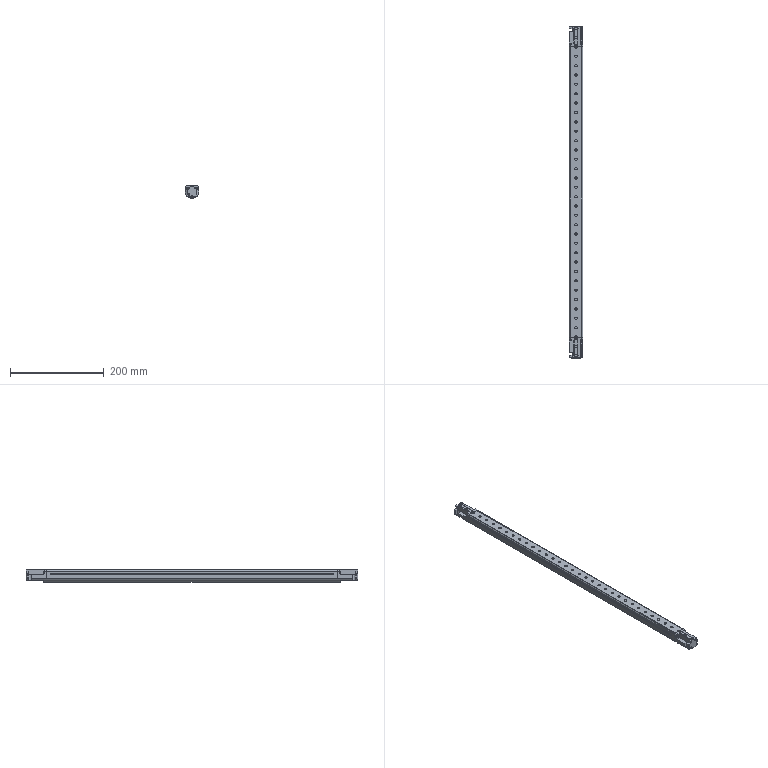Part | STEP file | Guide wheel mechanism revised.sldasm-Part-32 | 1 solid | 350 faces | box 28 x 710 x 26.2 mm | volume 446680 mm3 | cylinder 183 | plane 155 | spline 12 | commonest cylinder face diameters 5 x76 0.5 x12 3 x12 4.5 x12 4.9 x12 32 x11